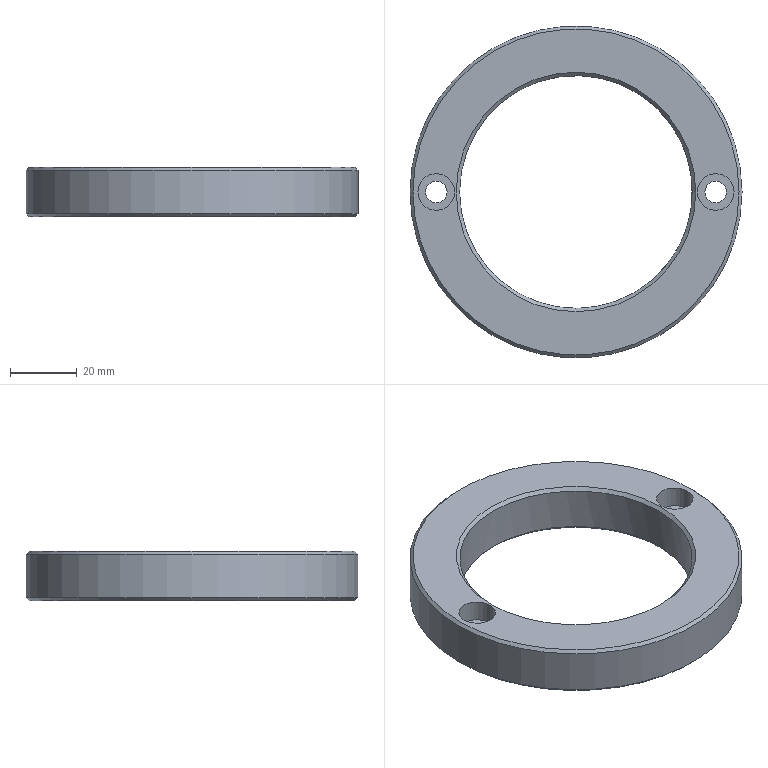Part | STEP file | lll_id158_x_t | 1 solid | 14 faces | box 99.8 x 99.8 x 15 mm | volume 57338 mm3 | cylinder 6 | plane 4 | cone 4 | commonest cylinder face diameters 6.5 x2 11 x2 70 x1 99.8 x1
STEP:
#1=CARTESIAN_POINT('',(49.,0.,165.5));
#2=VERTEX_POINT('',#1);
#3=CARTESIAN_POINT('',(0.,0.,165.5));
#4=DIRECTION('',(0.,0.,1.));
#5=DIRECTION('',(1.,0.,0.));
#6=AXIS2_PLACEMENT_3D('',#3,#4,#5);
#7=CIRCLE('',#6,49.);
#8=EDGE_CURVE('',#2,#2,#7,.T.);
#9=ORIENTED_EDGE('',*,*,#8,.T.);
#10=EDGE_LOOP('',(#9));
#11=FACE_BOUND('',#10,.T.);
#12=CARTESIAN_POINT('',(36.,0.,165.5));
#13=VERTEX_POINT('',#12);
#14=CARTESIAN_POINT('',(0.,0.,165.5));
#15=DIRECTION('',(0.,0.,-1.));
#16=DIRECTION('',(1.,0.,0.));
#17=AXIS2_PLACEMENT_3D('',#14,#15,#16);
#18=CIRCLE('',#17,36.);
#19=EDGE_CURVE('',#13,#13,#18,.T.);
#20=ORIENTED_EDGE('',*,*,#19,.T.);
#21=EDGE_LOOP('',(#20));
#22=FACE_BOUND('',#21,.T.);
#23=CARTESIAN_POINT('',(-36.5,0.,165.5));
#24=VERTEX_POINT('',#23);
#25=CARTESIAN_POINT('',(-42.,0.,165.5));
#26=DIRECTION('',(0.,0.,-1.));
#27=DIRECTION('',(1.,0.,0.));
#28=AXIS2_PLACEMENT_3D('',#25,#26,#27);
#29=CIRCLE('',#28,5.5);
#30=EDGE_CURVE('',#24,#24,#29,.T.);
#31=ORIENTED_EDGE('',*,*,#30,.T.);
#32=EDGE_LOOP('',(#31));
#33=FACE_BOUND('',#32,.T.);
#34=CARTESIAN_POINT('',(36.5,0.,165.5));
#35=VERTEX_POINT('',#34);
#36=CARTESIAN_POINT('',(42.,0.,165.5));
#37=DIRECTION('',(0.,0.,-1.));
#38=DIRECTION('',(-1.,0.,0.));
#39=AXIS2_PLACEMENT_3D('',#36,#37,#38);
#40=CIRCLE('',#39,5.5);
#41=EDGE_CURVE('',#35,#35,#40,.T.);
#42=ORIENTED_EDGE('',*,*,#41,.T.);
#43=EDGE_LOOP('',(#42));
#44=FACE_BOUND('',#43,.T.);
#45=CARTESIAN_POINT('',(0.,0.,165.5));
#46=DIRECTION('',(0.,0.,1.));
#47=DIRECTION('',(1.,0.,0.));
#48=AXIS2_PLACEMENT_3D('',#45,#46,#47);
#49=PLANE('',#48);
#50=ADVANCED_FACE('',(#11,#22,#33,#44),#49,.T.);
#51=CARTESIAN_POINT('',(-49.,0.,150.5));
#52=VERTEX_POINT('',#51);
#53=CARTESIAN_POINT('',(0.,0.,150.5));
#54=DIRECTION('',(0.,0.,-1.));
#55=DIRECTION('',(-1.,0.,0.));
#56=AXIS2_PLACEMENT_3D('',#53,#54,#55);
#57=CIRCLE('',#56,49.);
#58=EDGE_CURVE('',#52,#52,#57,.T.);
#59=ORIENTED_EDGE('',*,*,#58,.T.);
#60=EDGE_LOOP('',(#59));
#61=FACE_BOUND('',#60,.T.);
#62=CARTESIAN_POINT('',(-36.,0.,150.5));
#63=VERTEX_POINT('',#62);
#64=CARTESIAN_POINT('',(0.,0.,150.5));
#65=DIRECTION('',(0.,0.,1.));
#66=DIRECTION('',(-1.,0.,0.));
#67=AXIS2_PLACEMENT_3D('',#64,#65,#66);
#68=CIRCLE('',#67,36.);
#69=EDGE_CURVE('',#63,#63,#68,.T.);
#70=ORIENTED_EDGE('',*,*,#69,.T.);
#71=EDGE_LOOP('',(#70));
#72=FACE_BOUND('',#71,.T.);
#73=CARTESIAN_POINT('',(-45.25,0.,150.5));
#74=VERTEX_POINT('',#73);
#75=CARTESIAN_POINT('',(-42.,0.,150.5));
#76=DIRECTION('',(0.,0.,-1.));
#77=DIRECTION('',(-1.,0.,0.));
#78=AXIS2_PLACEMENT_3D('',#75,#76,#77);
#79=CIRCLE('',#78,3.25);
#80=EDGE_CURVE('',#74,#74,#79,.T.);
#81=ORIENTED_EDGE('',*,*,#80,.F.);
#82=EDGE_LOOP('',(#81));
#83=FACE_BOUND('',#82,.T.);
#84=CARTESIAN_POINT('',(38.75,0.,150.5));
#85=VERTEX_POINT('',#84);
#86=CARTESIAN_POINT('',(42.,0.,150.5));
#87=DIRECTION('',(0.,0.,-1.));
#88=DIRECTION('',(-1.,0.,0.));
#89=AXIS2_PLACEMENT_3D('',#86,#87,#88);
#90=CIRCLE('',#89,3.25);
#91=EDGE_CURVE('',#85,#85,#90,.T.);
#92=ORIENTED_EDGE('',*,*,#91,.F.);
#93=EDGE_LOOP('',(#92));
#94=FACE_BOUND('',#93,.T.);
#95=CARTESIAN_POINT('',(0.,0.,150.5));
#96=DIRECTION('',(0.,0.,-1.));
#97=DIRECTION('',(-1.,0.,0.));
#98=AXIS2_PLACEMENT_3D('',#95,#96,#97);
#99=PLANE('',#98);
#100=ADVANCED_FACE('',(#61,#72,#83,#94),#99,.T.);
#101=CARTESIAN_POINT('',(49.9,0.,151.4));
#102=VERTEX_POINT('',#101);
#103=CARTESIAN_POINT('',(0.,0.,151.4));
#104=DIRECTION('',(0.,0.,1.));
#105=DIRECTION('',(1.,0.,0.));
#106=AXIS2_PLACEMENT_3D('',#103,#104,#105);
#107=CIRCLE('',#106,49.9);
#108=EDGE_CURVE('',#102,#102,#107,.T.);
#109=ORIENTED_EDGE('',*,*,#108,.T.);
#110=EDGE_LOOP('',(#109));
#111=FACE_BOUND('',#110,.T.);
#112=CARTESIAN_POINT('',(-49.9,0.,164.6));
#113=VERTEX_POINT('',#112);
#114=CARTESIAN_POINT('',(0.,0.,164.6));
#115=DIRECTION('',(0.,0.,-1.));
#116=DIRECTION('',(-1.,0.,0.));
#117=AXIS2_PLACEMENT_3D('',#114,#115,#116);
#118=CIRCLE('',#117,49.9);
#119=EDGE_CURVE('',#113,#113,#118,.T.);
#120=ORIENTED_EDGE('',*,*,#119,.T.);
#121=EDGE_LOOP('',(#120));
#122=FACE_BOUND('',#121,.T.);
#123=CARTESIAN_POINT('',(0.,0.,150.5));
#124=DIRECTION('',(0.,0.,1.));
#125=DIRECTION('',(1.,0.,0.));
#126=AXIS2_PLACEMENT_3D('',#123,#124,#125);
#127=CYLINDRICAL_SURFACE('',#126,49.9);
#128=ADVANCED_FACE('',(#111,#122),#127,.T.);
#129=CARTESIAN_POINT('',(-35.,0.,151.5));
#130=VERTEX_POINT('',#129);
#131=CARTESIAN_POINT('',(0.,0.,151.5));
#132=DIRECTION('',(0.,0.,-1.));
#133=DIRECTION('',(-1.,0.,0.));
#134=AXIS2_PLACEMENT_3D('',#131,#132,#133);
#135=CIRCLE('',#134,35.);
#136=EDGE_CURVE('',#130,#130,#135,.T.);
#137=ORIENTED_EDGE('',*,*,#136,.T.);
#138=EDGE_LOOP('',(#137));
#139=FACE_BOUND('',#138,.T.);
#140=CARTESIAN_POINT('',(35.,0.,164.5));
#141=VERTEX_POINT('',#140);
#142=CARTESIAN_POINT('',(0.,0.,164.5));
#143=DIRECTION('',(0.,0.,1.));
#144=DIRECTION('',(1.,0.,0.));
#145=AXIS2_PLACEMENT_3D('',#142,#143,#144);
#146=CIRCLE('',#145,35.);
#147=EDGE_CURVE('',#141,#141,#146,.T.);
#148=ORIENTED_EDGE('',*,*,#147,.T.);
#149=EDGE_LOOP('',(#148));
#150=FACE_BOUND('',#149,.T.);
#151=CARTESIAN_POINT('',(0.,0.,165.5));
#152=DIRECTION('',(0.,0.,-1.));
#153=DIRECTION('',(-1.,0.,0.));
#154=AXIS2_PLACEMENT_3D('',#151,#152,#153);
#155=CYLINDRICAL_SURFACE('',#154,35.);
#156=ADVANCED_FACE('',(#139,#150),#155,.F.);
#157=ORIENTED_EDGE('',*,*,#91,.T.);
#158=EDGE_LOOP('',(#157));
#159=FACE_BOUND('',#158,.T.);
#160=CARTESIAN_POINT('',(38.75,0.,159.));
#161=VERTEX_POINT('',#160);
#162=CARTESIAN_POINT('',(42.,0.,159.));
#163=DIRECTION('',(0.,0.,-1.));
#164=DIRECTION('',(-1.,0.,0.));
#165=AXIS2_PLACEMENT_3D('',#162,#163,#164);
#166=CIRCLE('',#165,3.25);
#167=EDGE_CURVE('',#161,#161,#166,.T.);
#168=ORIENTED_EDGE('',*,*,#167,.F.);
#169=EDGE_LOOP('',(#168));
#170=FACE_BOUND('',#169,.T.);
#171=CARTESIAN_POINT('',(42.,0.,-134.5));
#172=DIRECTION('',(0.,0.,-1.));
#173=DIRECTION('',(-1.,0.,0.));
#174=AXIS2_PLACEMENT_3D('',#171,#172,#173);
#175=CYLINDRICAL_SURFACE('',#174,3.25);
#176=ADVANCED_FACE('',(#159,#170),#175,.F.);
#177=ORIENTED_EDGE('',*,*,#167,.T.);
#178=EDGE_LOOP('',(#177));
#179=FACE_BOUND('',#178,.T.);
#180=CARTESIAN_POINT('',(36.5,0.,159.));
#181=VERTEX_POINT('',#180);
#182=CARTESIAN_POINT('',(42.,0.,159.));
#183=DIRECTION('',(0.,0.,-1.));
#184=DIRECTION('',(-1.,0.,0.));
#185=AXIS2_PLACEMENT_3D('',#182,#183,#184);
#186=CIRCLE('',#185,5.5);
#187=EDGE_CURVE('',#181,#181,#186,.T.);
#188=ORIENTED_EDGE('',*,*,#187,.F.);
#189=EDGE_LOOP('',(#188));
#190=FACE_BOUND('',#189,.T.);
#191=CARTESIAN_POINT('',(42.,0.,159.));
#192=DIRECTION('',(0.,0.,-1.));
#193=DIRECTION('',(-1.,0.,0.));
#194=AXIS2_PLACEMENT_3D('',#191,#192,#193);
#195=PLANE('',#194);
#196=ADVANCED_FACE('',(#179,#190),#195,.F.);
#197=ORIENTED_EDGE('',*,*,#187,.T.);
#198=EDGE_LOOP('',(#197));
#199=FACE_BOUND('',#198,.T.);
#200=ORIENTED_EDGE('',*,*,#41,.F.);
#201=EDGE_LOOP('',(#200));
#202=FACE_BOUND('',#201,.T.);
#203=CARTESIAN_POINT('',(42.,0.,165.5));
#204=DIRECTION('',(0.,0.,-1.));
#205=DIRECTION('',(-1.,0.,0.));
#206=AXIS2_PLACEMENT_3D('',#203,#204,#205);
#207=CYLINDRICAL_SURFACE('',#206,5.5);
#208=ADVANCED_FACE('',(#199,#202),#207,.F.);
#209=ORIENTED_EDGE('',*,*,#80,.T.);
#210=EDGE_LOOP('',(#209));
#211=FACE_BOUND('',#210,.T.);
#212=CARTESIAN_POINT('',(-38.75,0.,159.));
#213=VERTEX_POINT('',#212);
#214=CARTESIAN_POINT('',(-42.,0.,159.));
#215=DIRECTION('',(0.,0.,-1.));
#216=DIRECTION('',(1.,0.,0.));
#217=AXIS2_PLACEMENT_3D('',#214,#215,#216);
#218=CIRCLE('',#217,3.25);
#219=EDGE_CURVE('',#213,#213,#218,.T.);
#220=ORIENTED_EDGE('',*,*,#219,.F.);
#221=EDGE_LOOP('',(#220));
#222=FACE_BOUND('',#221,.T.);
#223=CARTESIAN_POINT('',(-42.,0.,-134.5));
#224=DIRECTION('',(0.,0.,-1.));
#225=DIRECTION('',(1.,0.,0.));
#226=AXIS2_PLACEMENT_3D('',#223,#224,#225);
#227=CYLINDRICAL_SURFACE('',#226,3.25);
#228=ADVANCED_FACE('',(#211,#222),#227,.F.);
#229=ORIENTED_EDGE('',*,*,#219,.T.);
#230=EDGE_LOOP('',(#229));
#231=FACE_BOUND('',#230,.T.);
#232=CARTESIAN_POINT('',(-36.5,0.,159.));
#233=VERTEX_POINT('',#232);
#234=CARTESIAN_POINT('',(-42.,0.,159.));
#235=DIRECTION('',(0.,0.,-1.));
#236=DIRECTION('',(1.,0.,0.));
#237=AXIS2_PLACEMENT_3D('',#234,#235,#236);
#238=CIRCLE('',#237,5.5);
#239=EDGE_CURVE('',#233,#233,#238,.T.);
#240=ORIENTED_EDGE('',*,*,#239,.F.);
#241=EDGE_LOOP('',(#240));
#242=FACE_BOUND('',#241,.T.);
#243=CARTESIAN_POINT('',(-42.,0.,159.));
#244=DIRECTION('',(0.,0.,-1.));
#245=DIRECTION('',(1.,0.,0.));
#246=AXIS2_PLACEMENT_3D('',#243,#244,#245);
#247=PLANE('',#246);
#248=ADVANCED_FACE('',(#231,#242),#247,.F.);
#249=ORIENTED_EDGE('',*,*,#239,.T.);
#250=EDGE_LOOP('',(#249));
#251=FACE_BOUND('',#250,.T.);
#252=ORIENTED_EDGE('',*,*,#30,.F.);
#253=EDGE_LOOP('',(#252));
#254=FACE_BOUND('',#253,.T.);
#255=CARTESIAN_POINT('',(-42.,0.,165.5));
#256=DIRECTION('',(0.,0.,-1.));
#257=DIRECTION('',(1.,0.,0.));
#258=AXIS2_PLACEMENT_3D('',#255,#256,#257);
#259=CYLINDRICAL_SURFACE('',#258,5.5);
#260=ADVANCED_FACE('',(#251,#254),#259,.F.);
#261=ORIENTED_EDGE('',*,*,#58,.F.);
#262=EDGE_LOOP('',(#261));
#263=FACE_BOUND('',#262,.T.);
#264=ORIENTED_EDGE('',*,*,#108,.F.);
#265=EDGE_LOOP('',(#264));
#266=FACE_BOUND('',#265,.T.);
#267=CARTESIAN_POINT('',(0.,0.,151.5));
#268=DIRECTION('',(0.,0.,1.));
#269=DIRECTION('',(1.,0.,0.));
#270=AXIS2_PLACEMENT_3D('',#267,#268,#269);
#271=CONICAL_SURFACE('',#270,50.,45.);
#272=ADVANCED_FACE('',(#263,#266),#271,.T.);
#273=ORIENTED_EDGE('',*,*,#69,.F.);
#274=EDGE_LOOP('',(#273));
#275=FACE_BOUND('',#274,.T.);
#276=ORIENTED_EDGE('',*,*,#136,.F.);
#277=EDGE_LOOP('',(#276));
#278=FACE_BOUND('',#277,.T.);
#279=CARTESIAN_POINT('',(0.,0.,151.5));
#280=DIRECTION('',(0.,0.,-1.));
#281=DIRECTION('',(-1.,0.,0.));
#282=AXIS2_PLACEMENT_3D('',#279,#280,#281);
#283=CONICAL_SURFACE('',#282,35.,45.);
#284=ADVANCED_FACE('',(#275,#278),#283,.F.);
#285=ORIENTED_EDGE('',*,*,#8,.F.);
#286=EDGE_LOOP('',(#285));
#287=FACE_BOUND('',#286,.T.);
#288=ORIENTED_EDGE('',*,*,#119,.F.);
#289=EDGE_LOOP('',(#288));
#290=FACE_BOUND('',#289,.T.);
#291=CARTESIAN_POINT('',(0.,0.,164.5));
#292=DIRECTION('',(0.,0.,-1.));
#293=DIRECTION('',(-1.,0.,0.));
#294=AXIS2_PLACEMENT_3D('',#291,#292,#293);
#295=CONICAL_SURFACE('',#294,50.,45.);
#296=ADVANCED_FACE('',(#287,#290),#295,.T.);
#297=ORIENTED_EDGE('',*,*,#19,.F.);
#298=EDGE_LOOP('',(#297));
#299=FACE_BOUND('',#298,.T.);
#300=ORIENTED_EDGE('',*,*,#147,.F.);
#301=EDGE_LOOP('',(#300));
#302=FACE_BOUND('',#301,.T.);
#303=CARTESIAN_POINT('',(0.,0.,164.5));
#304=DIRECTION('',(0.,0.,1.));
#305=DIRECTION('',(1.,0.,0.));
#306=AXIS2_PLACEMENT_3D('',#303,#304,#305);
#307=CONICAL_SURFACE('',#306,35.,45.);
#308=ADVANCED_FACE('',(#299,#302),#307,.F.);
#309=CLOSED_SHELL('',(#50,#100,#128,#156,#176,#196,#208,#228,#248,#260,#272,#284,#296,#308));
#310=MANIFOLD_SOLID_BREP('',#309);
#311=(LENGTH_UNIT()NAMED_UNIT(*)SI_UNIT(.MILLI.,.METRE.));
#312=UNCERTAINTY_MEASURE_WITH_UNIT(LENGTH_MEASURE(0.00002),#311,'','');
#313=(NAMED_UNIT(*)PLANE_ANGLE_UNIT()SI_UNIT($,.RADIAN.));
#314=PLANE_ANGLE_MEASURE_WITH_UNIT(PLANE_ANGLE_MEASURE(0.01745),#313);
#315=DIMENSIONAL_EXPONENTS(0.,0.,0.,0.,0.,0.,0.);
#316=(CONVERSION_BASED_UNIT('DEGREE',#314)NAMED_UNIT(#315)PLANE_ANGLE_UNIT());
#317=(NAMED_UNIT(*)SI_UNIT($,.STERADIAN.)SOLID_ANGLE_UNIT());
#318=(GEOMETRIC_REPRESENTATION_CONTEXT(3)GLOBAL_UNCERTAINTY_ASSIGNED_CONTEXT((#312))GLOBAL_UNIT_ASSIGNED_CONTEXT((#311,#316,#317))REPRESENTATION_CONTEXT('',''));
#319=ADVANCED_BREP_SHAPE_REPRESENTATION('',(#310),#318);